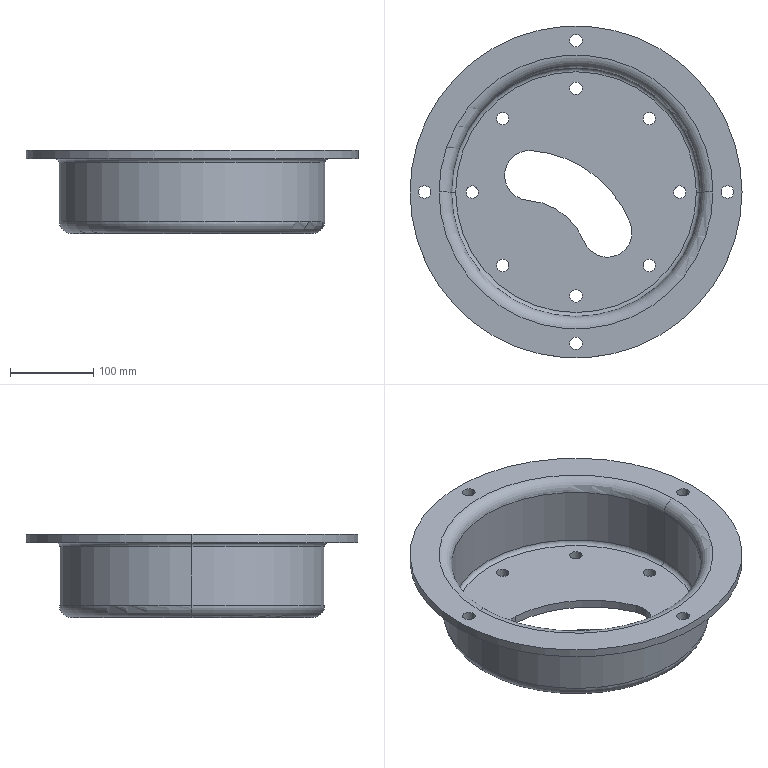Part | SolidWorks | features Fillet 2, ICE 2, Extrusion 1 | 1 solid | 47 faces | box 400 x 400 x 100 mm | volume 1926675 mm3 | cylinder 35 | torus 8 | plane 4 | commonest cylinder face diameters 15 x24 60 x3 300 x2 320 x2 400 x2 160 x1
STEP:
#1=CARTESIAN_POINT('',(-145.,0.,0.));
#2=VERTEX_POINT('',#1);
#3=CARTESIAN_POINT('',(145.,0.,0.));
#4=VERTEX_POINT('',#3);
#5=CARTESIAN_POINT('',(0.,0.,0.));
#6=DIRECTION('',(0.,0.,-1.));
#7=DIRECTION('',(1.,0.,0.));
#8=AXIS2_PLACEMENT_3D('',#5,#6,#7);
#9=CIRCLE('',#8,145.);
#10=EDGE_CURVE('',#2,#4,#9,.T.);
#11=ORIENTED_EDGE('',*,*,#10,.F.);
#12=CARTESIAN_POINT('',(-160.,0.,15.));
#13=VERTEX_POINT('',#12);
#14=CARTESIAN_POINT('',(-145.,0.,15.));
#15=DIRECTION('',(0.,1.,0.));
#16=DIRECTION('',(-1.,0.,0.));
#17=AXIS2_PLACEMENT_3D('',#14,#15,#16);
#18=CIRCLE('',#17,15.);
#19=EDGE_CURVE('',#2,#13,#18,.T.);
#20=ORIENTED_EDGE('',*,*,#19,.T.);
#21=CARTESIAN_POINT('',(160.,0.,15.));
#22=VERTEX_POINT('',#21);
#23=CARTESIAN_POINT('',(0.,0.,15.));
#24=DIRECTION('',(0.,0.,1.));
#25=DIRECTION('',(1.,0.,0.));
#26=AXIS2_PLACEMENT_3D('',#23,#24,#25);
#27=CIRCLE('',#26,160.);
#28=EDGE_CURVE('',#22,#13,#27,.T.);
#29=ORIENTED_EDGE('',*,*,#28,.F.);
#30=CARTESIAN_POINT('',(145.,0.,15.));
#31=DIRECTION('',(0.,-1.,0.));
#32=DIRECTION('',(0.,0.,-1.));
#33=AXIS2_PLACEMENT_3D('',#30,#31,#32);
#34=CIRCLE('',#33,15.);
#35=EDGE_CURVE('',#4,#22,#34,.T.);
#36=ORIENTED_EDGE('',*,*,#35,.F.);
#37=EDGE_LOOP('',(#11,#20,#29,#36));
#38=FACE_OUTER_BOUND('',#37,.T.);
#39=CARTESIAN_POINT('',(0.,0.,15.));
#40=DIRECTION('',(0.,0.,1.));
#41=DIRECTION('',(1.,0.,0.));
#42=AXIS2_PLACEMENT_3D('',#39,#40,#41);
#43=TOROIDAL_SURFACE('',#42,145.,15.);
#44=ADVANCED_FACE('',(#38),#43,.T.);
#45=CARTESIAN_POINT('',(-165.,0.,100.));
#46=VERTEX_POINT('',#45);
#47=CARTESIAN_POINT('',(165.,0.,100.));
#48=VERTEX_POINT('',#47);
#49=CARTESIAN_POINT('',(0.,0.,100.));
#50=DIRECTION('',(0.,0.,-1.));
#51=DIRECTION('',(1.,0.,0.));
#52=AXIS2_PLACEMENT_3D('',#49,#50,#51);
#53=CIRCLE('',#52,165.);
#54=EDGE_CURVE('',#46,#48,#53,.T.);
#55=ORIENTED_EDGE('',*,*,#54,.F.);
#56=CARTESIAN_POINT('',(-150.,0.,85.));
#57=VERTEX_POINT('',#56);
#58=CARTESIAN_POINT('',(-165.,0.,85.));
#59=DIRECTION('',(0.,1.,0.));
#60=DIRECTION('',(-1.,0.,0.));
#61=AXIS2_PLACEMENT_3D('',#58,#59,#60);
#62=CIRCLE('',#61,15.);
#63=EDGE_CURVE('',#46,#57,#62,.T.);
#64=ORIENTED_EDGE('',*,*,#63,.T.);
#65=CARTESIAN_POINT('',(150.,0.,85.));
#66=VERTEX_POINT('',#65);
#67=CARTESIAN_POINT('',(0.,0.,85.));
#68=DIRECTION('',(0.,0.,1.));
#69=DIRECTION('',(1.,0.,0.));
#70=AXIS2_PLACEMENT_3D('',#67,#68,#69);
#71=CIRCLE('',#70,150.);
#72=EDGE_CURVE('',#66,#57,#71,.T.);
#73=ORIENTED_EDGE('',*,*,#72,.F.);
#74=CARTESIAN_POINT('',(165.,0.,85.));
#75=DIRECTION('',(0.,-1.,0.));
#76=DIRECTION('',(0.,0.,-1.));
#77=AXIS2_PLACEMENT_3D('',#74,#75,#76);
#78=CIRCLE('',#77,15.);
#79=EDGE_CURVE('',#48,#66,#78,.T.);
#80=ORIENTED_EDGE('',*,*,#79,.F.);
#81=EDGE_LOOP('',(#55,#64,#73,#80));
#82=FACE_OUTER_BOUND('',#81,.T.);
#83=CARTESIAN_POINT('',(0.,0.,85.));
#84=DIRECTION('',(0.,0.,1.));
#85=DIRECTION('',(1.,0.,0.));
#86=AXIS2_PLACEMENT_3D('',#83,#84,#85);
#87=TOROIDAL_SURFACE('',#86,165.,15.);
#88=ADVANCED_FACE('',(#82),#87,.T.);
#89=CARTESIAN_POINT('',(-145.,0.,10.));
#90=VERTEX_POINT('',#89);
#91=CARTESIAN_POINT('',(145.,0.,10.));
#92=VERTEX_POINT('',#91);
#93=CARTESIAN_POINT('',(0.,0.,10.));
#94=DIRECTION('',(0.,0.,1.));
#95=DIRECTION('',(1.,0.,0.));
#96=AXIS2_PLACEMENT_3D('',#93,#94,#95);
#97=CIRCLE('',#96,145.);
#98=EDGE_CURVE('',#90,#92,#97,.T.);
#99=ORIENTED_EDGE('',*,*,#98,.F.);
#100=CARTESIAN_POINT('',(-150.,0.,15.));
#101=VERTEX_POINT('',#100);
#102=CARTESIAN_POINT('',(-145.,0.,15.));
#103=DIRECTION('',(0.,1.,0.));
#104=DIRECTION('',(-1.,0.,0.));
#105=AXIS2_PLACEMENT_3D('',#102,#103,#104);
#106=CIRCLE('',#105,5.);
#107=EDGE_CURVE('',#90,#101,#106,.T.);
#108=ORIENTED_EDGE('',*,*,#107,.T.);
#109=CARTESIAN_POINT('',(150.,0.,15.));
#110=VERTEX_POINT('',#109);
#111=CARTESIAN_POINT('',(0.,0.,15.));
#112=DIRECTION('',(0.,0.,-1.));
#113=DIRECTION('',(1.,0.,0.));
#114=AXIS2_PLACEMENT_3D('',#111,#112,#113);
#115=CIRCLE('',#114,150.);
#116=EDGE_CURVE('',#110,#101,#115,.T.);
#117=ORIENTED_EDGE('',*,*,#116,.F.);
#118=CARTESIAN_POINT('',(145.,0.,15.));
#119=DIRECTION('',(0.,-1.,0.));
#120=DIRECTION('',(0.,0.,-1.));
#121=AXIS2_PLACEMENT_3D('',#118,#119,#120);
#122=CIRCLE('',#121,5.);
#123=EDGE_CURVE('',#92,#110,#122,.T.);
#124=ORIENTED_EDGE('',*,*,#123,.F.);
#125=EDGE_LOOP('',(#99,#108,#117,#124));
#126=FACE_OUTER_BOUND('',#125,.T.);
#127=CARTESIAN_POINT('',(0.,0.,15.));
#128=DIRECTION('',(0.,0.,1.));
#129=DIRECTION('',(1.,0.,0.));
#130=AXIS2_PLACEMENT_3D('',#127,#128,#129);
#131=TOROIDAL_SURFACE('',#130,145.,5.);
#132=ADVANCED_FACE('',(#126),#131,.F.);
#133=CARTESIAN_POINT('',(-165.,0.,90.));
#134=VERTEX_POINT('',#133);
#135=CARTESIAN_POINT('',(165.,0.,90.));
#136=VERTEX_POINT('',#135);
#137=CARTESIAN_POINT('',(0.,0.,90.));
#138=DIRECTION('',(0.,0.,1.));
#139=DIRECTION('',(1.,0.,0.));
#140=AXIS2_PLACEMENT_3D('',#137,#138,#139);
#141=CIRCLE('',#140,165.);
#142=EDGE_CURVE('',#134,#136,#141,.T.);
#143=ORIENTED_EDGE('',*,*,#142,.F.);
#144=CARTESIAN_POINT('',(-160.,0.,85.));
#145=VERTEX_POINT('',#144);
#146=CARTESIAN_POINT('',(-165.,0.,85.));
#147=DIRECTION('',(0.,1.,0.));
#148=DIRECTION('',(-1.,0.,0.));
#149=AXIS2_PLACEMENT_3D('',#146,#147,#148);
#150=CIRCLE('',#149,5.);
#151=EDGE_CURVE('',#134,#145,#150,.T.);
#152=ORIENTED_EDGE('',*,*,#151,.T.);
#153=CARTESIAN_POINT('',(160.,0.,85.));
#154=VERTEX_POINT('',#153);
#155=CARTESIAN_POINT('',(0.,0.,85.));
#156=DIRECTION('',(0.,0.,-1.));
#157=DIRECTION('',(1.,0.,0.));
#158=AXIS2_PLACEMENT_3D('',#155,#156,#157);
#159=CIRCLE('',#158,160.);
#160=EDGE_CURVE('',#154,#145,#159,.T.);
#161=ORIENTED_EDGE('',*,*,#160,.F.);
#162=CARTESIAN_POINT('',(165.,0.,85.));
#163=DIRECTION('',(0.,-1.,0.));
#164=DIRECTION('',(0.,0.,-1.));
#165=AXIS2_PLACEMENT_3D('',#162,#163,#164);
#166=CIRCLE('',#165,5.);
#167=EDGE_CURVE('',#136,#154,#166,.T.);
#168=ORIENTED_EDGE('',*,*,#167,.F.);
#169=EDGE_LOOP('',(#143,#152,#161,#168));
#170=FACE_OUTER_BOUND('',#169,.T.);
#171=CARTESIAN_POINT('',(0.,0.,85.));
#172=DIRECTION('',(0.,0.,1.));
#173=DIRECTION('',(1.,0.,0.));
#174=AXIS2_PLACEMENT_3D('',#171,#172,#173);
#175=TOROIDAL_SURFACE('',#174,165.,5.);
#176=ADVANCED_FACE('',(#170),#175,.F.);
#177=CARTESIAN_POINT('',(-190.,0.,100.));
#178=VERTEX_POINT('',#177);
#179=CARTESIAN_POINT('',(-175.,0.,100.));
#180=VERTEX_POINT('',#179);
#181=CARTESIAN_POINT('',(-182.5,0.,100.));
#182=DIRECTION('',(0.,0.,1.));
#183=DIRECTION('',(1.,0.,0.));
#184=AXIS2_PLACEMENT_3D('',#181,#182,#183);
#185=CIRCLE('',#184,7.5);
#186=EDGE_CURVE('',#178,#180,#185,.T.);
#187=ORIENTED_EDGE('',*,*,#186,.T.);
#188=CARTESIAN_POINT('',(-175.,0.,90.));
#189=VERTEX_POINT('',#188);
#190=CARTESIAN_POINT('',(-175.,0.,100.));
#191=DIRECTION('',(0.,0.,-1.));
#192=VECTOR('',#191,1000.);
#193=LINE('',#190,#192);
#194=EDGE_CURVE('',#180,#189,#193,.T.);
#195=ORIENTED_EDGE('',*,*,#194,.T.);
#196=CARTESIAN_POINT('',(-190.,0.,90.));
#197=VERTEX_POINT('',#196);
#198=CARTESIAN_POINT('',(-182.5,0.,90.));
#199=DIRECTION('',(0.,0.,1.));
#200=DIRECTION('',(1.,0.,0.));
#201=AXIS2_PLACEMENT_3D('',#198,#199,#200);
#202=CIRCLE('',#201,7.5);
#203=EDGE_CURVE('',#197,#189,#202,.T.);
#204=ORIENTED_EDGE('',*,*,#203,.F.);
#205=CARTESIAN_POINT('',(-190.,0.,100.));
#206=DIRECTION('',(0.,0.,-1.));
#207=VECTOR('',#206,1000.);
#208=LINE('',#205,#207);
#209=EDGE_CURVE('',#178,#197,#208,.T.);
#210=ORIENTED_EDGE('',*,*,#209,.F.);
#211=EDGE_LOOP('',(#187,#195,#204,#210));
#212=FACE_OUTER_BOUND('',#211,.T.);
#213=CARTESIAN_POINT('',(-182.5,0.,100.));
#214=DIRECTION('',(0.,0.,-1.));
#215=DIRECTION('',(-1.,0.,0.));
#216=AXIS2_PLACEMENT_3D('',#213,#214,#215);
#217=CYLINDRICAL_SURFACE('',#216,7.5);
#218=ADVANCED_FACE('',(#212),#217,.F.);
#219=CARTESIAN_POINT('',(-7.5,-182.5,100.));
#220=VERTEX_POINT('',#219);
#221=CARTESIAN_POINT('',(7.5,-182.5,100.));
#222=VERTEX_POINT('',#221);
#223=CARTESIAN_POINT('',(0.,-182.5,100.));
#224=DIRECTION('',(0.,0.,1.));
#225=DIRECTION('',(1.,0.,0.));
#226=AXIS2_PLACEMENT_3D('',#223,#224,#225);
#227=CIRCLE('',#226,7.5);
#228=EDGE_CURVE('',#220,#222,#227,.T.);
#229=ORIENTED_EDGE('',*,*,#228,.T.);
#230=CARTESIAN_POINT('',(7.5,-182.5,90.));
#231=VERTEX_POINT('',#230);
#232=CARTESIAN_POINT('',(7.5,-182.5,100.));
#233=DIRECTION('',(0.,0.,-1.));
#234=VECTOR('',#233,1000.);
#235=LINE('',#232,#234);
#236=EDGE_CURVE('',#222,#231,#235,.T.);
#237=ORIENTED_EDGE('',*,*,#236,.T.);
#238=CARTESIAN_POINT('',(-7.5,-182.5,90.));
#239=VERTEX_POINT('',#238);
#240=CARTESIAN_POINT('',(0.,-182.5,90.));
#241=DIRECTION('',(0.,0.,1.));
#242=DIRECTION('',(1.,0.,0.));
#243=AXIS2_PLACEMENT_3D('',#240,#241,#242);
#244=CIRCLE('',#243,7.5);
#245=EDGE_CURVE('',#239,#231,#244,.T.);
#246=ORIENTED_EDGE('',*,*,#245,.F.);
#247=CARTESIAN_POINT('',(-7.5,-182.5,100.));
#248=DIRECTION('',(0.,0.,-1.));
#249=VECTOR('',#248,1000.);
#250=LINE('',#247,#249);
#251=EDGE_CURVE('',#220,#239,#250,.T.);
#252=ORIENTED_EDGE('',*,*,#251,.F.);
#253=EDGE_LOOP('',(#229,#237,#246,#252));
#254=FACE_OUTER_BOUND('',#253,.T.);
#255=CARTESIAN_POINT('',(0.,-182.5,100.));
#256=DIRECTION('',(0.,0.,-1.));
#257=DIRECTION('',(-1.,0.,0.));
#258=AXIS2_PLACEMENT_3D('',#255,#256,#257);
#259=CYLINDRICAL_SURFACE('',#258,7.5);
#260=ADVANCED_FACE('',(#254),#259,.F.);
#261=CARTESIAN_POINT('',(175.,0.,100.));
#262=VERTEX_POINT('',#261);
#263=CARTESIAN_POINT('',(190.,0.,100.));
#264=VERTEX_POINT('',#263);
#265=CARTESIAN_POINT('',(182.5,0.,100.));
#266=DIRECTION('',(0.,0.,1.));
#267=DIRECTION('',(1.,0.,0.));
#268=AXIS2_PLACEMENT_3D('',#265,#266,#267);
#269=CIRCLE('',#268,7.5);
#270=EDGE_CURVE('',#262,#264,#269,.T.);
#271=ORIENTED_EDGE('',*,*,#270,.T.);
#272=CARTESIAN_POINT('',(190.,0.,90.));
#273=VERTEX_POINT('',#272);
#274=CARTESIAN_POINT('',(190.,0.,100.));
#275=DIRECTION('',(0.,0.,-1.));
#276=VECTOR('',#275,1000.);
#277=LINE('',#274,#276);
#278=EDGE_CURVE('',#264,#273,#277,.T.);
#279=ORIENTED_EDGE('',*,*,#278,.T.);
#280=CARTESIAN_POINT('',(175.,0.,90.));
#281=VERTEX_POINT('',#280);
#282=CARTESIAN_POINT('',(182.5,0.,90.));
#283=DIRECTION('',(0.,0.,1.));
#284=DIRECTION('',(1.,0.,0.));
#285=AXIS2_PLACEMENT_3D('',#282,#283,#284);
#286=CIRCLE('',#285,7.5);
#287=EDGE_CURVE('',#281,#273,#286,.T.);
#288=ORIENTED_EDGE('',*,*,#287,.F.);
#289=CARTESIAN_POINT('',(175.,0.,100.));
#290=DIRECTION('',(0.,0.,-1.));
#291=VECTOR('',#290,1000.);
#292=LINE('',#289,#291);
#293=EDGE_CURVE('',#262,#281,#292,.T.);
#294=ORIENTED_EDGE('',*,*,#293,.F.);
#295=EDGE_LOOP('',(#271,#279,#288,#294));
#296=FACE_OUTER_BOUND('',#295,.T.);
#297=CARTESIAN_POINT('',(182.5,0.,100.));
#298=DIRECTION('',(0.,0.,-1.));
#299=DIRECTION('',(-1.,0.,0.));
#300=AXIS2_PLACEMENT_3D('',#297,#298,#299);
#301=CYLINDRICAL_SURFACE('',#300,7.5);
#302=ADVANCED_FACE('',(#296),#301,.F.);
#303=CARTESIAN_POINT('',(-7.5,182.5,100.));
#304=VERTEX_POINT('',#303);
#305=CARTESIAN_POINT('',(7.5,182.5,100.));
#306=VERTEX_POINT('',#305);
#307=CARTESIAN_POINT('',(0.,182.5,100.));
#308=DIRECTION('',(0.,0.,1.));
#309=DIRECTION('',(1.,0.,0.));
#310=AXIS2_PLACEMENT_3D('',#307,#308,#309);
#311=CIRCLE('',#310,7.5);
#312=EDGE_CURVE('',#304,#306,#311,.T.);
#313=ORIENTED_EDGE('',*,*,#312,.T.);
#314=CARTESIAN_POINT('',(7.5,182.5,90.));
#315=VERTEX_POINT('',#314);
#316=CARTESIAN_POINT('',(7.5,182.5,100.));
#317=DIRECTION('',(0.,0.,-1.));
#318=VECTOR('',#317,1000.);
#319=LINE('',#316,#318);
#320=EDGE_CURVE('',#306,#315,#319,.T.);
#321=ORIENTED_EDGE('',*,*,#320,.T.);
#322=CARTESIAN_POINT('',(-7.5,182.5,90.));
#323=VERTEX_POINT('',#322);
#324=CARTESIAN_POINT('',(0.,182.5,90.));
#325=DIRECTION('',(0.,0.,1.));
#326=DIRECTION('',(1.,0.,0.));
#327=AXIS2_PLACEMENT_3D('',#324,#325,#326);
#328=CIRCLE('',#327,7.5);
#329=EDGE_CURVE('',#323,#315,#328,.T.);
#330=ORIENTED_EDGE('',*,*,#329,.F.);
#331=CARTESIAN_POINT('',(-7.5,182.5,100.));
#332=DIRECTION('',(0.,0.,-1.));
#333=VECTOR('',#332,1000.);
#334=LINE('',#331,#333);
#335=EDGE_CURVE('',#304,#323,#334,.T.);
#336=ORIENTED_EDGE('',*,*,#335,.F.);
#337=EDGE_LOOP('',(#313,#321,#330,#336));
#338=FACE_OUTER_BOUND('',#337,.T.);
#339=CARTESIAN_POINT('',(0.,182.5,100.));
#340=DIRECTION('',(0.,0.,-1.));
#341=DIRECTION('',(-1.,0.,0.));
#342=AXIS2_PLACEMENT_3D('',#339,#340,#341);
#343=CYLINDRICAL_SURFACE('',#342,7.5);
#344=ADVANCED_FACE('',(#338),#343,.F.);
#345=CARTESIAN_POINT('',(200.,0.,100.));
#346=VERTEX_POINT('',#345);
#347=CARTESIAN_POINT('',(-200.,0.,100.));
#348=VERTEX_POINT('',#347);
#349=CARTESIAN_POINT('',(0.,0.,100.));
#350=DIRECTION('',(0.,0.,1.));
#351=DIRECTION('',(1.,0.,0.));
#352=AXIS2_PLACEMENT_3D('',#349,#350,#351);
#353=CIRCLE('',#352,200.);
#354=EDGE_CURVE('',#346,#348,#353,.T.);
#355=ORIENTED_EDGE('',*,*,#354,.F.);
#356=CARTESIAN_POINT('',(200.,0.,90.));
#357=VERTEX_POINT('',#356);
#358=CARTESIAN_POINT('',(200.,0.,100.));
#359=DIRECTION('',(0.,0.,-1.));
#360=VECTOR('',#359,1000.);
#361=LINE('',#358,#360);
#362=EDGE_CURVE('',#346,#357,#361,.T.);
#363=ORIENTED_EDGE('',*,*,#362,.T.);
#364=CARTESIAN_POINT('',(-200.,0.,90.));
#365=VERTEX_POINT('',#364);
#366=CARTESIAN_POINT('',(0.,0.,90.));
#367=DIRECTION('',(0.,0.,1.));
#368=DIRECTION('',(1.,0.,0.));
#369=AXIS2_PLACEMENT_3D('',#366,#367,#368);
#370=CIRCLE('',#369,200.);
#371=EDGE_CURVE('',#357,#365,#370,.T.);
#372=ORIENTED_EDGE('',*,*,#371,.T.);
#373=CARTESIAN_POINT('',(-200.,0.,100.));
#374=DIRECTION('',(0.,0.,-1.));
#375=VECTOR('',#374,1000.);
#376=LINE('',#373,#375);
#377=EDGE_CURVE('',#348,#365,#376,.T.);
#378=ORIENTED_EDGE('',*,*,#377,.F.);
#379=EDGE_LOOP('',(#355,#363,#372,#378));
#380=FACE_OUTER_BOUND('',#379,.T.);
#381=CARTESIAN_POINT('',(0.,0.,100.));
#382=DIRECTION('',(0.,0.,-1.));
#383=DIRECTION('',(-1.,0.,0.));
#384=AXIS2_PLACEMENT_3D('',#381,#382,#383);
#385=CYLINDRICAL_SURFACE('',#384,200.);
#386=ADVANCED_FACE('',(#380),#385,.T.);
#387=CARTESIAN_POINT('',(0.,0.,85.));
#388=DIRECTION('',(0.,0.,1.));
#389=DIRECTION('',(1.,0.,0.));
#390=AXIS2_PLACEMENT_3D('',#387,#388,#389);
#391=CIRCLE('',#390,150.);
#392=EDGE_CURVE('',#57,#66,#391,.T.);
#393=ORIENTED_EDGE('',*,*,#392,.T.);
#394=CARTESIAN_POINT('',(150.,0.,90.));
#395=DIRECTION('',(0.,0.,-1.));
#396=VECTOR('',#395,1000.);
#397=LINE('',#394,#396);
#398=EDGE_CURVE('',#66,#110,#397,.T.);
#399=ORIENTED_EDGE('',*,*,#398,.T.);
#400=ORIENTED_EDGE('',*,*,#116,.T.);
#401=CARTESIAN_POINT('',(-150.,0.,90.));
#402=DIRECTION('',(0.,0.,-1.));
#403=VECTOR('',#402,1000.);
#404=LINE('',#401,#403);
#405=EDGE_CURVE('',#57,#101,#404,.T.);
#406=ORIENTED_EDGE('',*,*,#405,.F.);
#407=EDGE_LOOP('',(#393,#399,#400,#406));
#408=FACE_OUTER_BOUND('',#407,.T.);
#409=CARTESIAN_POINT('',(0.,0.,90.));
#410=DIRECTION('',(0.,0.,-1.));
#411=DIRECTION('',(-1.,0.,0.));
#412=AXIS2_PLACEMENT_3D('',#409,#410,#411);
#413=CYLINDRICAL_SURFACE('',#412,150.);
#414=ADVANCED_FACE('',(#408),#413,.F.);
#415=CARTESIAN_POINT('',(-53.803,50.038,10.));
#416=VERTEX_POINT('',#415);
#417=CARTESIAN_POINT('',(-86.087,20.125,10.));
#418=VERTEX_POINT('',#417);
#419=CARTESIAN_POINT('',(-56.087,20.125,10.));
#420=DIRECTION('',(0.,0.,1.));
#421=DIRECTION('',(1.,0.,0.));
#422=AXIS2_PLACEMENT_3D('',#419,#420,#421);
#423=CIRCLE('',#422,30.);
#424=EDGE_CURVE('',#416,#418,#423,.T.);
#425=ORIENTED_EDGE('',*,*,#424,.T.);
#426=CARTESIAN_POINT('',(-86.087,20.125,0.));
#427=VERTEX_POINT('',#426);
#428=CARTESIAN_POINT('',(-86.087,20.125,10.));
#429=DIRECTION('',(0.,0.,-1.));
#430=VECTOR('',#429,1000.);
#431=LINE('',#428,#430);
#432=EDGE_CURVE('',#418,#427,#431,.T.);
#433=ORIENTED_EDGE('',*,*,#432,.T.);
#434=CARTESIAN_POINT('',(-53.803,50.038,0.));
#435=VERTEX_POINT('',#434);
#436=CARTESIAN_POINT('',(-56.087,20.125,0.));
#437=DIRECTION('',(0.,0.,1.));
#438=DIRECTION('',(1.,0.,0.));
#439=AXIS2_PLACEMENT_3D('',#436,#437,#438);
#440=CIRCLE('',#439,30.);
#441=EDGE_CURVE('',#435,#427,#440,.T.);
#442=ORIENTED_EDGE('',*,*,#441,.F.);
#443=CARTESIAN_POINT('',(-53.803,50.038,10.));
#444=DIRECTION('',(0.,0.,-1.));
#445=VECTOR('',#444,1000.);
#446=LINE('',#443,#445);
#447=EDGE_CURVE('',#416,#435,#446,.T.);
#448=ORIENTED_EDGE('',*,*,#447,.F.);
#449=EDGE_LOOP('',(#425,#433,#442,#448));
#450=FACE_OUTER_BOUND('',#449,.T.);
#451=CARTESIAN_POINT('',(-56.087,20.125,10.));
#452=DIRECTION('',(0.,0.,-1.));
#453=DIRECTION('',(-1.,0.,0.));
#454=AXIS2_PLACEMENT_3D('',#451,#452,#453);
#455=CYLINDRICAL_SURFACE('',#454,30.);
#456=ADVANCED_FACE('',(#450),#455,.F.);
#457=CARTESIAN_POINT('',(-95.888,88.388,10.));
#458=VERTEX_POINT('',#457);
#459=CARTESIAN_POINT('',(-80.888,88.388,10.));
#460=VERTEX_POINT('',#459);
#461=CARTESIAN_POINT('',(-88.388,88.388,10.));
#462=DIRECTION('',(0.,0.,1.));
#463=DIRECTION('',(1.,0.,0.));
#464=AXIS2_PLACEMENT_3D('',#461,#462,#463);
#465=CIRCLE('',#464,7.5);
#466=EDGE_CURVE('',#458,#460,#465,.T.);
#467=ORIENTED_EDGE('',*,*,#466,.T.);
#468=CARTESIAN_POINT('',(-80.888,88.388,0.));
#469=VERTEX_POINT('',#468);
#470=CARTESIAN_POINT('',(-80.888,88.388,10.));
#471=DIRECTION('',(0.,0.,-1.));
#472=VECTOR('',#471,1000.);
#473=LINE('',#470,#472);
#474=EDGE_CURVE('',#460,#469,#473,.T.);
#475=ORIENTED_EDGE('',*,*,#474,.T.);
#476=CARTESIAN_POINT('',(-95.888,88.388,0.));
#477=VERTEX_POINT('',#476);
#478=CARTESIAN_POINT('',(-88.388,88.388,0.));
#479=DIRECTION('',(0.,0.,1.));
#480=DIRECTION('',(1.,0.,0.));
#481=AXIS2_PLACEMENT_3D('',#478,#479,#480);
#482=CIRCLE('',#481,7.5);
#483=EDGE_CURVE('',#477,#469,#482,.T.);
#484=ORIENTED_EDGE('',*,*,#483,.F.);
#485=CARTESIAN_POINT('',(-95.888,88.388,10.));
#486=DIRECTION('',(0.,0.,-1.));
#487=VECTOR('',#486,1000.);
#488=LINE('',#485,#487);
#489=EDGE_CURVE('',#458,#477,#488,.T.);
#490=ORIENTED_EDGE('',*,*,#489,.F.);
#491=EDGE_LOOP('',(#467,#475,#484,#490));
#492=FACE_OUTER_BOUND('',#491,.T.);
#493=CARTESIAN_POINT('',(-88.388,88.388,10.));
#494=DIRECTION('',(0.,0.,-1.));
#495=DIRECTION('',(-1.,0.,0.));
#496=AXIS2_PLACEMENT_3D('',#493,#494,#495);
#497=CYLINDRICAL_SURFACE('',#496,7.5);
#498=ADVANCED_FACE('',(#492),#497,.F.);
#499=CARTESIAN_POINT('',(-132.5,0.,10.));
#500=VERTEX_POINT('',#499);
#501=CARTESIAN_POINT('',(-117.5,0.,10.));
#502=VERTEX_POINT('',#501);
#503=CARTESIAN_POINT('',(-125.,0.,10.));
#504=DIRECTION('',(0.,0.,1.));
#505=DIRECTION('',(1.,0.,0.));
#506=AXIS2_PLACEMENT_3D('',#503,#504,#505);
#507=CIRCLE('',#506,7.5);
#508=EDGE_CURVE('',#500,#502,#507,.T.);
#509=ORIENTED_EDGE('',*,*,#508,.T.);
#510=CARTESIAN_POINT('',(-117.5,0.,0.));
#511=VERTEX_POINT('',#510);
#512=CARTESIAN_POINT('',(-117.5,0.,10.));
#513=DIRECTION('',(0.,0.,-1.));
#514=VECTOR('',#513,1000.);
#515=LINE('',#512,#514);
#516=EDGE_CURVE('',#502,#511,#515,.T.);
#517=ORIENTED_EDGE('',*,*,#516,.T.);
#518=CARTESIAN_POINT('',(-132.5,0.,0.));
#519=VERTEX_POINT('',#518);
#520=CARTESIAN_POINT('',(-125.,0.,0.));
#521=DIRECTION('',(0.,0.,1.));
#522=DIRECTION('',(1.,0.,0.));
#523=AXIS2_PLACEMENT_3D('',#520,#521,#522);
#524=CIRCLE('',#523,7.5);
#525=EDGE_CURVE('',#519,#511,#524,.T.);
#526=ORIENTED_EDGE('',*,*,#525,.F.);
#527=CARTESIAN_POINT('',(-132.5,0.,10.));
#528=DIRECTION('',(0.,0.,-1.));
#529=VECTOR('',#528,1000.);
#530=LINE('',#527,#529);
#531=EDGE_CURVE('',#500,#519,#530,.T.);
#532=ORIENTED_EDGE('',*,*,#531,.F.);
#533=EDGE_LOOP('',(#509,#517,#526,#532));
#534=FACE_OUTER_BOUND('',#533,.T.);
#535=CARTESIAN_POINT('',(-125.,0.,10.));
#536=DIRECTION('',(0.,0.,-1.));
#537=DIRECTION('',(-1.,0.,0.));
#538=AXIS2_PLACEMENT_3D('',#535,#536,#537);
#539=CYLINDRICAL_SURFACE('',#538,7.5);
#540=ADVANCED_FACE('',(#534),#539,.F.);
#541=CARTESIAN_POINT('',(-95.888,-88.388,10.));
#542=VERTEX_POINT('',#541);
#543=CARTESIAN_POINT('',(-80.888,-88.388,10.));
#544=VERTEX_POINT('',#543);
#545=CARTESIAN_POINT('',(-88.388,-88.388,10.));
#546=DIRECTION('',(0.,0.,1.));
#547=DIRECTION('',(1.,0.,0.));
#548=AXIS2_PLACEMENT_3D('',#545,#546,#547);
#549=CIRCLE('',#548,7.5);
#550=EDGE_CURVE('',#542,#544,#549,.T.);
#551=ORIENTED_EDGE('',*,*,#550,.T.);
#552=CARTESIAN_POINT('',(-80.888,-88.388,0.));
#553=VERTEX_POINT('',#552);
#554=CARTESIAN_POINT('',(-80.888,-88.388,10.));
#555=DIRECTION('',(0.,0.,-1.));
#556=VECTOR('',#555,1000.);
#557=LINE('',#554,#556);
#558=EDGE_CURVE('',#544,#553,#557,.T.);
#559=ORIENTED_EDGE('',*,*,#558,.T.);
#560=CARTESIAN_POINT('',(-95.888,-88.388,0.));
#561=VERTEX_POINT('',#560);
#562=CARTESIAN_POINT('',(-88.388,-88.388,0.));
#563=DIRECTION('',(0.,0.,1.));
#564=DIRECTION('',(1.,0.,0.));
#565=AXIS2_PLACEMENT_3D('',#562,#563,#564);
#566=CIRCLE('',#565,7.5);
#567=EDGE_CURVE('',#561,#553,#566,.T.);
#568=ORIENTED_EDGE('',*,*,#567,.F.);
#569=CARTESIAN_POINT('',(-95.888,-88.388,10.));
#570=DIRECTION('',(0.,0.,-1.));
#571=VECTOR('',#570,1000.);
#572=LINE('',#569,#571);
#573=EDGE_CURVE('',#542,#561,#572,.T.);
#574=ORIENTED_EDGE('',*,*,#573,.F.);
#575=EDGE_LOOP('',(#551,#559,#568,#574));
#576=FACE_OUTER_BOUND('',#575,.T.);
#577=CARTESIAN_POINT('',(-88.388,-88.388,10.));
#578=DIRECTION('',(0.,0.,-1.));
#579=DIRECTION('',(-1.,0.,0.));
#580=AXIS2_PLACEMENT_3D('',#577,#578,#579);
#581=CYLINDRICAL_SURFACE('',#580,7.5);
#582=ADVANCED_FACE('',(#576),#581,.F.);
#583=CARTESIAN_POINT('',(-7.5,-125.,10.));
#584=VERTEX_POINT('',#583);
#585=CARTESIAN_POINT('',(7.5,-125.,10.));
#586=VERTEX_POINT('',#585);
#587=CARTESIAN_POINT('',(0.,-125.,10.));
#588=DIRECTION('',(0.,0.,1.));
#589=DIRECTION('',(1.,0.,0.));
#590=AXIS2_PLACEMENT_3D('',#587,#588,#589);
#591=CIRCLE('',#590,7.5);
#592=EDGE_CURVE('',#584,#586,#591,.T.);
#593=ORIENTED_EDGE('',*,*,#592,.T.);
#594=CARTESIAN_POINT('',(7.5,-125.,0.));
#595=VERTEX_POINT('',#594);
#596=CARTESIAN_POINT('',(7.5,-125.,10.));
#597=DIRECTION('',(0.,0.,-1.));
#598=VECTOR('',#597,1000.);
#599=LINE('',#596,#598);
#600=EDGE_CURVE('',#586,#595,#599,.T.);
#601=ORIENTED_EDGE('',*,*,#600,.T.);
#602=CARTESIAN_POINT('',(-7.5,-125.,0.));
#603=VERTEX_POINT('',#602);
#604=CARTESIAN_POINT('',(0.,-125.,0.));
#605=DIRECTION('',(0.,0.,1.));
#606=DIRECTION('',(1.,0.,0.));
#607=AXIS2_PLACEMENT_3D('',#604,#605,#606);
#608=CIRCLE('',#607,7.5);
#609=EDGE_CURVE('',#603,#595,#608,.T.);
#610=ORIENTED_EDGE('',*,*,#609,.F.);
#611=CARTESIAN_POINT('',(-7.5,-125.,10.));
#612=DIRECTION('',(0.,0.,-1.));
#613=VECTOR('',#612,1000.);
#614=LINE('',#611,#613);
#615=EDGE_CURVE('',#584,#603,#614,.T.);
#616=ORIENTED_EDGE('',*,*,#615,.F.);
#617=EDGE_LOOP('',(#593,#601,#610,#616));
#618=FACE_OUTER_BOUND('',#617,.T.);
#619=CARTESIAN_POINT('',(0.,-125.,10.));
#620=DIRECTION('',(0.,0.,-1.));
#621=DIRECTION('',(-1.,0.,0.));
#622=AXIS2_PLACEMENT_3D('',#619,#620,#621);
#623=CYLINDRICAL_SURFACE('',#622,7.5);
#624=ADVANCED_FACE('',(#618),#623,.F.);
#625=CARTESIAN_POINT('',(80.888,-88.388,10.));
#626=VERTEX_POINT('',#625);
#627=CARTESIAN_POINT('',(95.888,-88.388,10.));
#628=VERTEX_POINT('',#627);
#629=CARTESIAN_POINT('',(88.388,-88.388,10.));
#630=DIRECTION('',(0.,0.,1.));
#631=DIRECTION('',(1.,0.,0.));
#632=AXIS2_PLACEMENT_3D('',#629,#630,#631);
#633=CIRCLE('',#632,7.5);
#634=EDGE_CURVE('',#626,#628,#633,.T.);
#635=ORIENTED_EDGE('',*,*,#634,.T.);
#636=CARTESIAN_POINT('',(95.888,-88.388,0.));
#637=VERTEX_POINT('',#636);
#638=CARTESIAN_POINT('',(95.888,-88.388,10.));
#639=DIRECTION('',(0.,0.,-1.));
#640=VECTOR('',#639,1000.);
#641=LINE('',#638,#640);
#642=EDGE_CURVE('',#628,#637,#641,.T.);
#643=ORIENTED_EDGE('',*,*,#642,.T.);
#644=CARTESIAN_POINT('',(80.888,-88.388,0.));
#645=VERTEX_POINT('',#644);
#646=CARTESIAN_POINT('',(88.388,-88.388,0.));
#647=DIRECTION('',(0.,0.,1.));
#648=DIRECTION('',(1.,0.,0.));
#649=AXIS2_PLACEMENT_3D('',#646,#647,#648);
#650=CIRCLE('',#649,7.5);
#651=EDGE_CURVE('',#645,#637,#650,.T.);
#652=ORIENTED_EDGE('',*,*,#651,.F.);
#653=CARTESIAN_POINT('',(80.888,-88.388,10.));
#654=DIRECTION('',(0.,0.,-1.));
#655=VECTOR('',#654,1000.);
#656=LINE('',#653,#655);
#657=EDGE_CURVE('',#626,#645,#656,.T.);
#658=ORIENTED_EDGE('',*,*,#657,.F.);
#659=EDGE_LOOP('',(#635,#643,#652,#658));
#660=FACE_OUTER_BOUND('',#659,.T.);
#661=CARTESIAN_POINT('',(88.388,-88.388,10.));
#662=DIRECTION('',(0.,0.,-1.));
#663=DIRECTION('',(-1.,0.,0.));
#664=AXIS2_PLACEMENT_3D('',#661,#662,#663);
#665=CYLINDRICAL_SURFACE('',#664,7.5);
#666=ADVANCED_FACE('',(#660),#665,.F.);
#667=CARTESIAN_POINT('',(117.5,0.,10.));
#668=VERTEX_POINT('',#667);
#669=CARTESIAN_POINT('',(132.5,0.,10.));
#670=VERTEX_POINT('',#669);
#671=CARTESIAN_POINT('',(125.,0.,10.));
#672=DIRECTION('',(0.,0.,1.));
#673=DIRECTION('',(1.,0.,0.));
#674=AXIS2_PLACEMENT_3D('',#671,#672,#673);
#675=CIRCLE('',#674,7.5);
#676=EDGE_CURVE('',#668,#670,#675,.T.);
#677=ORIENTED_EDGE('',*,*,#676,.T.);
#678=CARTESIAN_POINT('',(132.5,0.,0.));
#679=VERTEX_POINT('',#678);
#680=CARTESIAN_POINT('',(132.5,0.,10.));
#681=DIRECTION('',(0.,0.,-1.));
#682=VECTOR('',#681,1000.);
#683=LINE('',#680,#682);
#684=EDGE_CURVE('',#670,#679,#683,.T.);
#685=ORIENTED_EDGE('',*,*,#684,.T.);
#686=CARTESIAN_POINT('',(117.5,0.,0.));
#687=VERTEX_POINT('',#686);
#688=CARTESIAN_POINT('',(125.,0.,0.));
#689=DIRECTION('',(0.,0.,1.));
#690=DIRECTION('',(1.,0.,0.));
#691=AXIS2_PLACEMENT_3D('',#688,#689,#690);
#692=CIRCLE('',#691,7.5);
#693=EDGE_CURVE('',#687,#679,#692,.T.);
#694=ORIENTED_EDGE('',*,*,#693,.F.);
#695=CARTESIAN_POINT('',(117.5,0.,10.));
#696=DIRECTION('',(0.,0.,-1.));
#697=VECTOR('',#696,1000.);
#698=LINE('',#695,#697);
#699=EDGE_CURVE('',#668,#687,#698,.T.);
#700=ORIENTED_EDGE('',*,*,#699,.F.);
#701=EDGE_LOOP('',(#677,#685,#694,#700));
#702=FACE_OUTER_BOUND('',#701,.T.);
#703=CARTESIAN_POINT('',(125.,0.,10.));
#704=DIRECTION('',(0.,0.,-1.));
#705=DIRECTION('',(-1.,0.,0.));
#706=AXIS2_PLACEMENT_3D('',#703,#704,#705);
#707=CYLINDRICAL_SURFACE('',#706,7.5);
#708=ADVANCED_FACE('',(#702),#707,.F.);
#709=CARTESIAN_POINT('',(80.888,88.388,10.));
#710=VERTEX_POINT('',#709);
#711=CARTESIAN_POINT('',(95.888,88.388,10.));
#712=VERTEX_POINT('',#711);
#713=CARTESIAN_POINT('',(88.388,88.388,10.));
#714=DIRECTION('',(0.,0.,1.));
#715=DIRECTION('',(1.,0.,0.));
#716=AXIS2_PLACEMENT_3D('',#713,#714,#715);
#717=CIRCLE('',#716,7.5);
#718=EDGE_CURVE('',#710,#712,#717,.T.);
#719=ORIENTED_EDGE('',*,*,#718,.T.);
#720=CARTESIAN_POINT('',(95.888,88.388,0.));
#721=VERTEX_POINT('',#720);
#722=CARTESIAN_POINT('',(95.888,88.388,10.));
#723=DIRECTION('',(0.,0.,-1.));
#724=VECTOR('',#723,1000.);
#725=LINE('',#722,#724);
#726=EDGE_CURVE('',#712,#721,#725,.T.);
#727=ORIENTED_EDGE('',*,*,#726,.T.);
#728=CARTESIAN_POINT('',(80.888,88.388,0.));
#729=VERTEX_POINT('',#728);
#730=CARTESIAN_POINT('',(88.388,88.388,0.));
#731=DIRECTION('',(0.,0.,1.));
#732=DIRECTION('',(1.,0.,0.));
#733=AXIS2_PLACEMENT_3D('',#730,#731,#732);
#734=CIRCLE('',#733,7.5);
#735=EDGE_CURVE('',#729,#721,#734,.T.);
#736=ORIENTED_EDGE('',*,*,#735,.F.);
#737=CARTESIAN_POINT('',(80.888,88.388,10.));
#738=DIRECTION('',(0.,0.,-1.));
#739=VECTOR('',#738,1000.);
#740=LINE('',#737,#739);
#741=EDGE_CURVE('',#710,#729,#740,.T.);
#742=ORIENTED_EDGE('',*,*,#741,.F.);
#743=EDGE_LOOP('',(#719,#727,#736,#742));
#744=FACE_OUTER_BOUND('',#743,.T.);
#745=CARTESIAN_POINT('',(88.388,88.388,10.));
#746=DIRECTION('',(0.,0.,-1.));
#747=DIRECTION('',(-1.,0.,0.));
#748=AXIS2_PLACEMENT_3D('',#745,#746,#747);
#749=CYLINDRICAL_SURFACE('',#748,7.5);
#750=ADVANCED_FACE('',(#744),#749,.F.);
#751=CARTESIAN_POINT('',(-7.5,125.,10.));
#752=VERTEX_POINT('',#751);
#753=CARTESIAN_POINT('',(7.5,125.,10.));
#754=VERTEX_POINT('',#753);
#755=CARTESIAN_POINT('',(0.,125.,10.));
#756=DIRECTION('',(0.,0.,1.));
#757=DIRECTION('',(1.,0.,0.));
#758=AXIS2_PLACEMENT_3D('',#755,#756,#757);
#759=CIRCLE('',#758,7.5);
#760=EDGE_CURVE('',#752,#754,#759,.T.);
#761=ORIENTED_EDGE('',*,*,#760,.T.);
#762=CARTESIAN_POINT('',(7.5,125.,0.));
#763=VERTEX_POINT('',#762);
#764=CARTESIAN_POINT('',(7.5,125.,10.));
#765=DIRECTION('',(0.,0.,-1.));
#766=VECTOR('',#765,1000.);
#767=LINE('',#764,#766);
#768=EDGE_CURVE('',#754,#763,#767,.T.);
#769=ORIENTED_EDGE('',*,*,#768,.T.);
#770=CARTESIAN_POINT('',(-7.5,125.,0.));
#771=VERTEX_POINT('',#770);
#772=CARTESIAN_POINT('',(0.,125.,0.));
#773=DIRECTION('',(0.,0.,1.));
#774=DIRECTION('',(1.,0.,0.));
#775=AXIS2_PLACEMENT_3D('',#772,#773,#774);
#776=CIRCLE('',#775,7.5);
#777=EDGE_CURVE('',#771,#763,#776,.T.);
#778=ORIENTED_EDGE('',*,*,#777,.F.);
#779=CARTESIAN_POINT('',(-7.5,125.,10.));
#780=DIRECTION('',(0.,0.,-1.));
#781=VECTOR('',#780,1000.);
#782=LINE('',#779,#781);
#783=EDGE_CURVE('',#752,#771,#782,.T.);
#784=ORIENTED_EDGE('',*,*,#783,.F.);
#785=EDGE_LOOP('',(#761,#769,#778,#784));
#786=FACE_OUTER_BOUND('',#785,.T.);
#787=CARTESIAN_POINT('',(0.,125.,10.));
#788=DIRECTION('',(0.,0.,-1.));
#789=DIRECTION('',(-1.,0.,0.));
#790=AXIS2_PLACEMENT_3D('',#787,#788,#789);
#791=CYLINDRICAL_SURFACE('',#790,7.5);
#792=ADVANCED_FACE('',(#786),#791,.F.);
#793=CARTESIAN_POINT('',(0.,0.,85.));
#794=DIRECTION('',(0.,0.,-1.));
#795=DIRECTION('',(1.,0.,0.));
#796=AXIS2_PLACEMENT_3D('',#793,#794,#795);
#797=CIRCLE('',#796,160.);
#798=EDGE_CURVE('',#145,#154,#797,.T.);
#799=ORIENTED_EDGE('',*,*,#798,.T.);
#800=CARTESIAN_POINT('',(160.,0.,10.));
#801=DIRECTION('',(0.,0.,-1.));
#802=VECTOR('',#801,1000.);
#803=LINE('',#800,#802);
#804=EDGE_CURVE('',#154,#22,#803,.T.);
#805=ORIENTED_EDGE('',*,*,#804,.T.);
#806=ORIENTED_EDGE('',*,*,#28,.T.);
#807=CARTESIAN_POINT('',(-160.,0.,10.));
#808=DIRECTION('',(0.,0.,-1.));
#809=VECTOR('',#808,1000.);
#810=LINE('',#807,#809);
#811=EDGE_CURVE('',#145,#13,#810,.T.);
#812=ORIENTED_EDGE('',*,*,#811,.F.);
#813=EDGE_LOOP('',(#799,#805,#806,#812));
#814=FACE_OUTER_BOUND('',#813,.T.);
#815=CARTESIAN_POINT('',(0.,0.,10.));
#816=DIRECTION('',(0.,0.,-1.));
#817=DIRECTION('',(-1.,0.,0.));
#818=AXIS2_PLACEMENT_3D('',#815,#816,#817);
#819=CYLINDRICAL_SURFACE('',#818,160.);
#820=ADVANCED_FACE('',(#814),#819,.T.);
#821=CARTESIAN_POINT('',(0.,0.,10.));
#822=DIRECTION('',(0.,0.,1.));
#823=DIRECTION('',(1.,0.,0.));
#824=AXIS2_PLACEMENT_3D('',#821,#822,#823);
#825=CIRCLE('',#824,145.);
#826=EDGE_CURVE('',#92,#90,#825,.T.);
#827=ORIENTED_EDGE('',*,*,#826,.T.);
#828=ORIENTED_EDGE('',*,*,#98,.T.);
#829=EDGE_LOOP('',(#827,#828));
#830=FACE_OUTER_BOUND('',#829,.T.);
#831=CARTESIAN_POINT('',(9.752,-59.684,10.));
#832=VERTEX_POINT('',#831);
#833=CARTESIAN_POINT('',(65.412,-37.281,10.));
#834=VERTEX_POINT('',#833);
#835=CARTESIAN_POINT('',(37.582,-48.482,10.));
#836=DIRECTION('',(0.,0.,1.));
#837=DIRECTION('',(1.,0.,0.));
#838=AXIS2_PLACEMENT_3D('',#835,#836,#837);
#839=CIRCLE('',#838,30.);
#840=EDGE_CURVE('',#832,#834,#839,.T.);
#841=ORIENTED_EDGE('',*,*,#840,.F.);
#842=CARTESIAN_POINT('',(-58.371,-9.788,10.));
#843=VERTEX_POINT('',#842);
#844=CARTESIAN_POINT('',(-64.462,-89.556,10.));
#845=DIRECTION('',(0.,0.,-1.));
#846=DIRECTION('',(1.,0.,0.));
#847=AXIS2_PLACEMENT_3D('',#844,#845,#846);
#848=CIRCLE('',#847,80.);
#849=EDGE_CURVE('',#843,#832,#848,.T.);
#850=ORIENTED_EDGE('',*,*,#849,.F.);
#851=CARTESIAN_POINT('',(-56.087,20.125,10.));
#852=DIRECTION('',(0.,0.,1.));
#853=DIRECTION('',(1.,0.,0.));
#854=AXIS2_PLACEMENT_3D('',#851,#852,#853);
#855=CIRCLE('',#854,30.);
#856=EDGE_CURVE('',#418,#843,#855,.T.);
#857=ORIENTED_EDGE('',*,*,#856,.F.);
#858=ORIENTED_EDGE('',*,*,#424,.F.);
#859=CARTESIAN_POINT('',(-64.462,-89.556,10.));
#860=DIRECTION('',(0.,0.,1.));
#861=DIRECTION('',(1.,0.,0.));
#862=AXIS2_PLACEMENT_3D('',#859,#860,#861);
#863=CIRCLE('',#862,140.);
#864=EDGE_CURVE('',#834,#416,#863,.T.);
#865=ORIENTED_EDGE('',*,*,#864,.F.);
#866=EDGE_LOOP('',(#841,#850,#857,#858,#865));
#867=FACE_BOUND('',#866,.T.);
#868=ORIENTED_EDGE('',*,*,#466,.F.);
#869=CARTESIAN_POINT('',(-88.388,88.388,10.));
#870=DIRECTION('',(0.,0.,1.));
#871=DIRECTION('',(1.,0.,0.));
#872=AXIS2_PLACEMENT_3D('',#869,#870,#871);
#873=CIRCLE('',#872,7.5);
#874=EDGE_CURVE('',#460,#458,#873,.T.);
#875=ORIENTED_EDGE('',*,*,#874,.F.);
#876=EDGE_LOOP('',(#868,#875));
#877=FACE_BOUND('',#876,.T.);
#878=ORIENTED_EDGE('',*,*,#550,.F.);
#879=CARTESIAN_POINT('',(-88.388,-88.388,10.));
#880=DIRECTION('',(0.,0.,1.));
#881=DIRECTION('',(1.,0.,0.));
#882=AXIS2_PLACEMENT_3D('',#879,#880,#881);
#883=CIRCLE('',#882,7.5);
#884=EDGE_CURVE('',#544,#542,#883,.T.);
#885=ORIENTED_EDGE('',*,*,#884,.F.);
#886=EDGE_LOOP('',(#878,#885));
#887=FACE_BOUND('',#886,.T.);
#888=ORIENTED_EDGE('',*,*,#634,.F.);
#889=CARTESIAN_POINT('',(88.388,-88.388,10.));
#890=DIRECTION('',(0.,0.,1.));
#891=DIRECTION('',(1.,0.,0.));
#892=AXIS2_PLACEMENT_3D('',#889,#890,#891);
#893=CIRCLE('',#892,7.5);
#894=EDGE_CURVE('',#628,#626,#893,.T.);
#895=ORIENTED_EDGE('',*,*,#894,.F.);
#896=EDGE_LOOP('',(#888,#895));
#897=FACE_BOUND('',#896,.T.);
#898=ORIENTED_EDGE('',*,*,#718,.F.);
#899=CARTESIAN_POINT('',(88.388,88.388,10.));
#900=DIRECTION('',(0.,0.,1.));
#901=DIRECTION('',(1.,0.,0.));
#902=AXIS2_PLACEMENT_3D('',#899,#900,#901);
#903=CIRCLE('',#902,7.5);
#904=EDGE_CURVE('',#712,#710,#903,.T.);
#905=ORIENTED_EDGE('',*,*,#904,.F.);
#906=EDGE_LOOP('',(#898,#905));
#907=FACE_BOUND('',#906,.T.);
#908=ORIENTED_EDGE('',*,*,#760,.F.);
#909=CARTESIAN_POINT('',(0.,125.,10.));
#910=DIRECTION('',(0.,0.,1.));
#911=DIRECTION('',(1.,0.,0.));
#912=AXIS2_PLACEMENT_3D('',#909,#910,#911);
#913=CIRCLE('',#912,7.5);
#914=EDGE_CURVE('',#754,#752,#913,.T.);
#915=ORIENTED_EDGE('',*,*,#914,.F.);
#916=EDGE_LOOP('',(#908,#915));
#917=FACE_BOUND('',#916,.T.);
#918=ORIENTED_EDGE('',*,*,#676,.F.);
#919=CARTESIAN_POINT('',(125.,0.,10.));
#920=DIRECTION('',(0.,0.,1.));
#921=DIRECTION('',(1.,0.,0.));
#922=AXIS2_PLACEMENT_3D('',#919,#920,#921);
#923=CIRCLE('',#922,7.5);
#924=EDGE_CURVE('',#670,#668,#923,.T.);
#925=ORIENTED_EDGE('',*,*,#924,.F.);
#926=EDGE_LOOP('',(#918,#925));
#927=FACE_BOUND('',#926,.T.);
#928=ORIENTED_EDGE('',*,*,#592,.F.);
#929=CARTESIAN_POINT('',(0.,-125.,10.));
#930=DIRECTION('',(0.,0.,1.));
#931=DIRECTION('',(1.,0.,0.));
#932=AXIS2_PLACEMENT_3D('',#929,#930,#931);
#933=CIRCLE('',#932,7.5);
#934=EDGE_CURVE('',#586,#584,#933,.T.);
#935=ORIENTED_EDGE('',*,*,#934,.F.);
#936=EDGE_LOOP('',(#928,#935));
#937=FACE_BOUND('',#936,.T.);
#938=ORIENTED_EDGE('',*,*,#508,.F.);
#939=CARTESIAN_POINT('',(-125.,0.,10.));
#940=DIRECTION('',(0.,0.,1.));
#941=DIRECTION('',(1.,0.,0.));
#942=AXIS2_PLACEMENT_3D('',#939,#940,#941);
#943=CIRCLE('',#942,7.5);
#944=EDGE_CURVE('',#502,#500,#943,.T.);
#945=ORIENTED_EDGE('',*,*,#944,.F.);
#946=EDGE_LOOP('',(#938,#945));
#947=FACE_BOUND('',#946,.T.);
#948=CARTESIAN_POINT('',(0.,0.,10.));
#949=DIRECTION('',(0.,0.,1.));
#950=DIRECTION('',(1.,0.,0.));
#951=AXIS2_PLACEMENT_3D('',#948,#949,#950);
#952=PLANE('',#951);
#953=ADVANCED_FACE('',(#830,#867,#877,#887,#897,#907,#917,#927,#937,#947),#952,.T.);
#954=CARTESIAN_POINT('',(0.,0.,0.));
#955=DIRECTION('',(0.,0.,-1.));
#956=DIRECTION('',(1.,0.,0.));
#957=AXIS2_PLACEMENT_3D('',#954,#955,#956);
#958=CIRCLE('',#957,145.);
#959=EDGE_CURVE('',#4,#2,#958,.T.);
#960=ORIENTED_EDGE('',*,*,#959,.T.);
#961=ORIENTED_EDGE('',*,*,#10,.T.);
#962=EDGE_LOOP('',(#960,#961));
#963=FACE_OUTER_BOUND('',#962,.T.);
#964=ORIENTED_EDGE('',*,*,#483,.T.);
#965=CARTESIAN_POINT('',(-88.388,88.388,0.));
#966=DIRECTION('',(0.,0.,1.));
#967=DIRECTION('',(1.,0.,0.));
#968=AXIS2_PLACEMENT_3D('',#965,#966,#967);
#969=CIRCLE('',#968,7.5);
#970=EDGE_CURVE('',#469,#477,#969,.T.);
#971=ORIENTED_EDGE('',*,*,#970,.T.);
#972=EDGE_LOOP('',(#964,#971));
#973=FACE_BOUND('',#972,.T.);
#974=ORIENTED_EDGE('',*,*,#525,.T.);
#975=CARTESIAN_POINT('',(-125.,0.,0.));
#976=DIRECTION('',(0.,0.,1.));
#977=DIRECTION('',(1.,0.,0.));
#978=AXIS2_PLACEMENT_3D('',#975,#976,#977);
#979=CIRCLE('',#978,7.5);
#980=EDGE_CURVE('',#511,#519,#979,.T.);
#981=ORIENTED_EDGE('',*,*,#980,.T.);
#982=EDGE_LOOP('',(#974,#981));
#983=FACE_BOUND('',#982,.T.);
#984=ORIENTED_EDGE('',*,*,#567,.T.);
#985=CARTESIAN_POINT('',(-88.388,-88.388,0.));
#986=DIRECTION('',(0.,0.,1.));
#987=DIRECTION('',(1.,0.,0.));
#988=AXIS2_PLACEMENT_3D('',#985,#986,#987);
#989=CIRCLE('',#988,7.5);
#990=EDGE_CURVE('',#553,#561,#989,.T.);
#991=ORIENTED_EDGE('',*,*,#990,.T.);
#992=EDGE_LOOP('',(#984,#991));
#993=FACE_BOUND('',#992,.T.);
#994=ORIENTED_EDGE('',*,*,#609,.T.);
#995=CARTESIAN_POINT('',(0.,-125.,0.));
#996=DIRECTION('',(0.,0.,1.));
#997=DIRECTION('',(1.,0.,0.));
#998=AXIS2_PLACEMENT_3D('',#995,#996,#997);
#999=CIRCLE('',#998,7.5);
#1000=EDGE_CURVE('',#595,#603,#999,.T.);
#1001=ORIENTED_EDGE('',*,*,#1000,.T.);
#1002=EDGE_LOOP('',(#994,#1001));
#1003=FACE_BOUND('',#1002,.T.);
#1004=ORIENTED_EDGE('',*,*,#651,.T.);
#1005=CARTESIAN_POINT('',(88.388,-88.388,0.));
#1006=DIRECTION('',(0.,0.,1.));
#1007=DIRECTION('',(1.,0.,0.));
#1008=AXIS2_PLACEMENT_3D('',#1005,#1006,#1007);
#1009=CIRCLE('',#1008,7.5);
#1010=EDGE_CURVE('',#637,#645,#1009,.T.);
#1011=ORIENTED_EDGE('',*,*,#1010,.T.);
#1012=EDGE_LOOP('',(#1004,#1011));
#1013=FACE_BOUND('',#1012,.T.);
#1014=ORIENTED_EDGE('',*,*,#693,.T.);
#1015=CARTESIAN_POINT('',(125.,0.,0.));
#1016=DIRECTION('',(0.,0.,1.));
#1017=DIRECTION('',(1.,0.,0.));
#1018=AXIS2_PLACEMENT_3D('',#1015,#1016,#1017);
#1019=CIRCLE('',#1018,7.5);
#1020=EDGE_CURVE('',#679,#687,#1019,.T.);
#1021=ORIENTED_EDGE('',*,*,#1020,.T.);
#1022=EDGE_LOOP('',(#1014,#1021));
#1023=FACE_BOUND('',#1022,.T.);
#1024=ORIENTED_EDGE('',*,*,#735,.T.);
#1025=CARTESIAN_POINT('',(88.388,88.388,0.));
#1026=DIRECTION('',(0.,0.,1.));
#1027=DIRECTION('',(1.,0.,0.));
#1028=AXIS2_PLACEMENT_3D('',#1025,#1026,#1027);
#1029=CIRCLE('',#1028,7.5);
#1030=EDGE_CURVE('',#721,#729,#1029,.T.);
#1031=ORIENTED_EDGE('',*,*,#1030,.T.);
#1032=EDGE_LOOP('',(#1024,#1031));
#1033=FACE_BOUND('',#1032,.T.);
#1034=ORIENTED_EDGE('',*,*,#777,.T.);
#1035=CARTESIAN_POINT('',(0.,125.,0.));
#1036=DIRECTION('',(0.,0.,1.));
#1037=DIRECTION('',(1.,0.,0.));
#1038=AXIS2_PLACEMENT_3D('',#1035,#1036,#1037);
#1039=CIRCLE('',#1038,7.5);
#1040=EDGE_CURVE('',#763,#771,#1039,.T.);
#1041=ORIENTED_EDGE('',*,*,#1040,.T.);
#1042=EDGE_LOOP('',(#1034,#1041));
#1043=FACE_BOUND('',#1042,.T.);
#1044=CARTESIAN_POINT('',(-58.371,-9.788,0.));
#1045=VERTEX_POINT('',#1044);
#1046=CARTESIAN_POINT('',(9.752,-59.684,0.));
#1047=VERTEX_POINT('',#1046);
#1048=CARTESIAN_POINT('',(-64.462,-89.556,0.));
#1049=DIRECTION('',(0.,0.,-1.));
#1050=DIRECTION('',(1.,0.,0.));
#1051=AXIS2_PLACEMENT_3D('',#1048,#1049,#1050);
#1052=CIRCLE('',#1051,80.);
#1053=EDGE_CURVE('',#1045,#1047,#1052,.T.);
#1054=ORIENTED_EDGE('',*,*,#1053,.T.);
#1055=CARTESIAN_POINT('',(65.412,-37.281,0.));
#1056=VERTEX_POINT('',#1055);
#1057=CARTESIAN_POINT('',(37.582,-48.482,0.));
#1058=DIRECTION('',(0.,0.,1.));
#1059=DIRECTION('',(1.,0.,0.));
#1060=AXIS2_PLACEMENT_3D('',#1057,#1058,#1059);
#1061=CIRCLE('',#1060,30.);
#1062=EDGE_CURVE('',#1047,#1056,#1061,.T.);
#1063=ORIENTED_EDGE('',*,*,#1062,.T.);
#1064=CARTESIAN_POINT('',(-64.462,-89.556,0.));
#1065=DIRECTION('',(0.,0.,1.));
#1066=DIRECTION('',(1.,0.,0.));
#1067=AXIS2_PLACEMENT_3D('',#1064,#1065,#1066);
#1068=CIRCLE('',#1067,140.);
#1069=EDGE_CURVE('',#1056,#435,#1068,.T.);
#1070=ORIENTED_EDGE('',*,*,#1069,.T.);
#1071=ORIENTED_EDGE('',*,*,#441,.T.);
#1072=CARTESIAN_POINT('',(-56.087,20.125,0.));
#1073=DIRECTION('',(0.,0.,1.));
#1074=DIRECTION('',(1.,0.,0.));
#1075=AXIS2_PLACEMENT_3D('',#1072,#1073,#1074);
#1076=CIRCLE('',#1075,30.);
#1077=EDGE_CURVE('',#427,#1045,#1076,.T.);
#1078=ORIENTED_EDGE('',*,*,#1077,.T.);
#1079=EDGE_LOOP('',(#1054,#1063,#1070,#1071,#1078));
#1080=FACE_BOUND('',#1079,.T.);
#1081=CARTESIAN_POINT('',(0.,0.,0.));
#1082=DIRECTION('',(0.,0.,1.));
#1083=DIRECTION('',(1.,0.,0.));
#1084=AXIS2_PLACEMENT_3D('',#1081,#1082,#1083);
#1085=PLANE('',#1084);
#1086=ADVANCED_FACE('',(#963,#973,#983,#993,#1003,#1013,#1023,#1033,#1043,#1080),#1085,.F.);
#1087=ORIENTED_EDGE('',*,*,#804,.F.);
#1088=ORIENTED_EDGE('',*,*,#160,.T.);
#1089=ORIENTED_EDGE('',*,*,#811,.T.);
#1090=CARTESIAN_POINT('',(0.,0.,15.));
#1091=DIRECTION('',(0.,0.,1.));
#1092=DIRECTION('',(1.,0.,0.));
#1093=AXIS2_PLACEMENT_3D('',#1090,#1091,#1092);
#1094=CIRCLE('',#1093,160.);
#1095=EDGE_CURVE('',#13,#22,#1094,.T.);
#1096=ORIENTED_EDGE('',*,*,#1095,.T.);
#1097=EDGE_LOOP('',(#1087,#1088,#1089,#1096));
#1098=FACE_OUTER_BOUND('',#1097,.T.);
#1099=CARTESIAN_POINT('',(0.,0.,10.));
#1100=DIRECTION('',(0.,0.,-1.));
#1101=DIRECTION('',(-1.,0.,0.));
#1102=AXIS2_PLACEMENT_3D('',#1099,#1100,#1101);
#1103=CYLINDRICAL_SURFACE('',#1102,160.);
#1104=ADVANCED_FACE('',(#1098),#1103,.T.);
#1105=ORIENTED_EDGE('',*,*,#768,.F.);
#1106=ORIENTED_EDGE('',*,*,#914,.T.);
#1107=ORIENTED_EDGE('',*,*,#783,.T.);
#1108=ORIENTED_EDGE('',*,*,#1040,.F.);
#1109=EDGE_LOOP('',(#1105,#1106,#1107,#1108));
#1110=FACE_OUTER_BOUND('',#1109,.T.);
#1111=CARTESIAN_POINT('',(0.,125.,10.));
#1112=DIRECTION('',(0.,0.,-1.));
#1113=DIRECTION('',(-1.,0.,0.));
#1114=AXIS2_PLACEMENT_3D('',#1111,#1112,#1113);
#1115=CYLINDRICAL_SURFACE('',#1114,7.5);
#1116=ADVANCED_FACE('',(#1110),#1115,.F.);
#1117=ORIENTED_EDGE('',*,*,#726,.F.);
#1118=ORIENTED_EDGE('',*,*,#904,.T.);
#1119=ORIENTED_EDGE('',*,*,#741,.T.);
#1120=ORIENTED_EDGE('',*,*,#1030,.F.);
#1121=EDGE_LOOP('',(#1117,#1118,#1119,#1120));
#1122=FACE_OUTER_BOUND('',#1121,.T.);
#1123=CARTESIAN_POINT('',(88.388,88.388,10.));
#1124=DIRECTION('',(0.,0.,-1.));
#1125=DIRECTION('',(-1.,0.,0.));
#1126=AXIS2_PLACEMENT_3D('',#1123,#1124,#1125);
#1127=CYLINDRICAL_SURFACE('',#1126,7.5);
#1128=ADVANCED_FACE('',(#1122),#1127,.F.);
#1129=ORIENTED_EDGE('',*,*,#684,.F.);
#1130=ORIENTED_EDGE('',*,*,#924,.T.);
#1131=ORIENTED_EDGE('',*,*,#699,.T.);
#1132=ORIENTED_EDGE('',*,*,#1020,.F.);
#1133=EDGE_LOOP('',(#1129,#1130,#1131,#1132));
#1134=FACE_OUTER_BOUND('',#1133,.T.);
#1135=CARTESIAN_POINT('',(125.,0.,10.));
#1136=DIRECTION('',(0.,0.,-1.));
#1137=DIRECTION('',(-1.,0.,0.));
#1138=AXIS2_PLACEMENT_3D('',#1135,#1136,#1137);
#1139=CYLINDRICAL_SURFACE('',#1138,7.5);
#1140=ADVANCED_FACE('',(#1134),#1139,.F.);
#1141=ORIENTED_EDGE('',*,*,#642,.F.);
#1142=ORIENTED_EDGE('',*,*,#894,.T.);
#1143=ORIENTED_EDGE('',*,*,#657,.T.);
#1144=ORIENTED_EDGE('',*,*,#1010,.F.);
#1145=EDGE_LOOP('',(#1141,#1142,#1143,#1144));
#1146=FACE_OUTER_BOUND('',#1145,.T.);
#1147=CARTESIAN_POINT('',(88.388,-88.388,10.));
#1148=DIRECTION('',(0.,0.,-1.));
#1149=DIRECTION('',(-1.,0.,0.));
#1150=AXIS2_PLACEMENT_3D('',#1147,#1148,#1149);
#1151=CYLINDRICAL_SURFACE('',#1150,7.5);
#1152=ADVANCED_FACE('',(#1146),#1151,.F.);
#1153=ORIENTED_EDGE('',*,*,#600,.F.);
#1154=ORIENTED_EDGE('',*,*,#934,.T.);
#1155=ORIENTED_EDGE('',*,*,#615,.T.);
#1156=ORIENTED_EDGE('',*,*,#1000,.F.);
#1157=EDGE_LOOP('',(#1153,#1154,#1155,#1156));
#1158=FACE_OUTER_BOUND('',#1157,.T.);
#1159=CARTESIAN_POINT('',(0.,-125.,10.));
#1160=DIRECTION('',(0.,0.,-1.));
#1161=DIRECTION('',(-1.,0.,0.));
#1162=AXIS2_PLACEMENT_3D('',#1159,#1160,#1161);
#1163=CYLINDRICAL_SURFACE('',#1162,7.5);
#1164=ADVANCED_FACE('',(#1158),#1163,.F.);
#1165=ORIENTED_EDGE('',*,*,#558,.F.);
#1166=ORIENTED_EDGE('',*,*,#884,.T.);
#1167=ORIENTED_EDGE('',*,*,#573,.T.);
#1168=ORIENTED_EDGE('',*,*,#990,.F.);
#1169=EDGE_LOOP('',(#1165,#1166,#1167,#1168));
#1170=FACE_OUTER_BOUND('',#1169,.T.);
#1171=CARTESIAN_POINT('',(-88.388,-88.388,10.));
#1172=DIRECTION('',(0.,0.,-1.));
#1173=DIRECTION('',(-1.,0.,0.));
#1174=AXIS2_PLACEMENT_3D('',#1171,#1172,#1173);
#1175=CYLINDRICAL_SURFACE('',#1174,7.5);
#1176=ADVANCED_FACE('',(#1170),#1175,.F.);
#1177=ORIENTED_EDGE('',*,*,#516,.F.);
#1178=ORIENTED_EDGE('',*,*,#944,.T.);
#1179=ORIENTED_EDGE('',*,*,#531,.T.);
#1180=ORIENTED_EDGE('',*,*,#980,.F.);
#1181=EDGE_LOOP('',(#1177,#1178,#1179,#1180));
#1182=FACE_OUTER_BOUND('',#1181,.T.);
#1183=CARTESIAN_POINT('',(-125.,0.,10.));
#1184=DIRECTION('',(0.,0.,-1.));
#1185=DIRECTION('',(-1.,0.,0.));
#1186=AXIS2_PLACEMENT_3D('',#1183,#1184,#1185);
#1187=CYLINDRICAL_SURFACE('',#1186,7.5);
#1188=ADVANCED_FACE('',(#1182),#1187,.F.);
#1189=ORIENTED_EDGE('',*,*,#474,.F.);
#1190=ORIENTED_EDGE('',*,*,#874,.T.);
#1191=ORIENTED_EDGE('',*,*,#489,.T.);
#1192=ORIENTED_EDGE('',*,*,#970,.F.);
#1193=EDGE_LOOP('',(#1189,#1190,#1191,#1192));
#1194=FACE_OUTER_BOUND('',#1193,.T.);
#1195=CARTESIAN_POINT('',(-88.388,88.388,10.));
#1196=DIRECTION('',(0.,0.,-1.));
#1197=DIRECTION('',(-1.,0.,0.));
#1198=AXIS2_PLACEMENT_3D('',#1195,#1196,#1197);
#1199=CYLINDRICAL_SURFACE('',#1198,7.5);
#1200=ADVANCED_FACE('',(#1194),#1199,.F.);
#1201=ORIENTED_EDGE('',*,*,#1053,.F.);
#1202=CARTESIAN_POINT('',(-58.371,-9.788,10.));
#1203=DIRECTION('',(0.,0.,-1.));
#1204=VECTOR('',#1203,1000.);
#1205=LINE('',#1202,#1204);
#1206=EDGE_CURVE('',#843,#1045,#1205,.T.);
#1207=ORIENTED_EDGE('',*,*,#1206,.F.);
#1208=ORIENTED_EDGE('',*,*,#849,.T.);
#1209=CARTESIAN_POINT('',(9.752,-59.684,10.));
#1210=DIRECTION('',(0.,0.,-1.));
#1211=VECTOR('',#1210,1000.);
#1212=LINE('',#1209,#1211);
#1213=EDGE_CURVE('',#832,#1047,#1212,.T.);
#1214=ORIENTED_EDGE('',*,*,#1213,.T.);
#1215=EDGE_LOOP('',(#1201,#1207,#1208,#1214));
#1216=FACE_OUTER_BOUND('',#1215,.T.);
#1217=CARTESIAN_POINT('',(-64.462,-89.556,10.));
#1218=DIRECTION('',(0.,0.,-1.));
#1219=DIRECTION('',(-1.,0.,0.));
#1220=AXIS2_PLACEMENT_3D('',#1217,#1218,#1219);
#1221=CYLINDRICAL_SURFACE('',#1220,80.);
#1222=ADVANCED_FACE('',(#1216),#1221,.T.);
#1223=ORIENTED_EDGE('',*,*,#1062,.F.);
#1224=ORIENTED_EDGE('',*,*,#1213,.F.);
#1225=ORIENTED_EDGE('',*,*,#840,.T.);
#1226=CARTESIAN_POINT('',(65.412,-37.281,10.));
#1227=DIRECTION('',(0.,0.,-1.));
#1228=VECTOR('',#1227,1000.);
#1229=LINE('',#1226,#1228);
#1230=EDGE_CURVE('',#834,#1056,#1229,.T.);
#1231=ORIENTED_EDGE('',*,*,#1230,.T.);
#1232=EDGE_LOOP('',(#1223,#1224,#1225,#1231));
#1233=FACE_OUTER_BOUND('',#1232,.T.);
#1234=CARTESIAN_POINT('',(37.582,-48.482,10.));
#1235=DIRECTION('',(0.,0.,-1.));
#1236=DIRECTION('',(-1.,0.,0.));
#1237=AXIS2_PLACEMENT_3D('',#1234,#1235,#1236);
#1238=CYLINDRICAL_SURFACE('',#1237,30.);
#1239=ADVANCED_FACE('',(#1233),#1238,.F.);
#1240=ORIENTED_EDGE('',*,*,#1069,.F.);
#1241=ORIENTED_EDGE('',*,*,#1230,.F.);
#1242=ORIENTED_EDGE('',*,*,#864,.T.);
#1243=ORIENTED_EDGE('',*,*,#447,.T.);
#1244=EDGE_LOOP('',(#1240,#1241,#1242,#1243));
#1245=FACE_OUTER_BOUND('',#1244,.T.);
#1246=CARTESIAN_POINT('',(-64.462,-89.556,10.));
#1247=DIRECTION('',(0.,0.,-1.));
#1248=DIRECTION('',(-1.,0.,0.));
#1249=AXIS2_PLACEMENT_3D('',#1246,#1247,#1248);
#1250=CYLINDRICAL_SURFACE('',#1249,140.);
#1251=ADVANCED_FACE('',(#1245),#1250,.F.);
#1252=ORIENTED_EDGE('',*,*,#432,.F.);
#1253=ORIENTED_EDGE('',*,*,#856,.T.);
#1254=ORIENTED_EDGE('',*,*,#1206,.T.);
#1255=ORIENTED_EDGE('',*,*,#1077,.F.);
#1256=EDGE_LOOP('',(#1252,#1253,#1254,#1255));
#1257=FACE_OUTER_BOUND('',#1256,.T.);
#1258=CARTESIAN_POINT('',(-56.087,20.125,10.));
#1259=DIRECTION('',(0.,0.,-1.));
#1260=DIRECTION('',(-1.,0.,0.));
#1261=AXIS2_PLACEMENT_3D('',#1258,#1259,#1260);
#1262=CYLINDRICAL_SURFACE('',#1261,30.);
#1263=ADVANCED_FACE('',(#1257),#1262,.F.);
#1264=ORIENTED_EDGE('',*,*,#398,.F.);
#1265=ORIENTED_EDGE('',*,*,#72,.T.);
#1266=ORIENTED_EDGE('',*,*,#405,.T.);
#1267=CARTESIAN_POINT('',(0.,0.,15.));
#1268=DIRECTION('',(0.,0.,-1.));
#1269=DIRECTION('',(1.,0.,0.));
#1270=AXIS2_PLACEMENT_3D('',#1267,#1268,#1269);
#1271=CIRCLE('',#1270,150.);
#1272=EDGE_CURVE('',#101,#110,#1271,.T.);
#1273=ORIENTED_EDGE('',*,*,#1272,.T.);
#1274=EDGE_LOOP('',(#1264,#1265,#1266,#1273));
#1275=FACE_OUTER_BOUND('',#1274,.T.);
#1276=CARTESIAN_POINT('',(0.,0.,90.));
#1277=DIRECTION('',(0.,0.,-1.));
#1278=DIRECTION('',(-1.,0.,0.));
#1279=AXIS2_PLACEMENT_3D('',#1276,#1277,#1278);
#1280=CYLINDRICAL_SURFACE('',#1279,150.);
#1281=ADVANCED_FACE('',(#1275),#1280,.F.);
#1282=CARTESIAN_POINT('',(0.,0.,100.));
#1283=DIRECTION('',(0.,0.,-1.));
#1284=DIRECTION('',(1.,0.,0.));
#1285=AXIS2_PLACEMENT_3D('',#1282,#1283,#1284);
#1286=CIRCLE('',#1285,165.);
#1287=EDGE_CURVE('',#48,#46,#1286,.T.);
#1288=ORIENTED_EDGE('',*,*,#1287,.T.);
#1289=ORIENTED_EDGE('',*,*,#54,.T.);
#1290=EDGE_LOOP('',(#1288,#1289));
#1291=FACE_BOUND('',#1290,.T.);
#1292=ORIENTED_EDGE('',*,*,#228,.F.);
#1293=CARTESIAN_POINT('',(0.,-182.5,100.));
#1294=DIRECTION('',(0.,0.,1.));
#1295=DIRECTION('',(1.,0.,0.));
#1296=AXIS2_PLACEMENT_3D('',#1293,#1294,#1295);
#1297=CIRCLE('',#1296,7.5);
#1298=EDGE_CURVE('',#222,#220,#1297,.T.);
#1299=ORIENTED_EDGE('',*,*,#1298,.F.);
#1300=EDGE_LOOP('',(#1292,#1299));
#1301=FACE_BOUND('',#1300,.T.);
#1302=ORIENTED_EDGE('',*,*,#312,.F.);
#1303=CARTESIAN_POINT('',(0.,182.5,100.));
#1304=DIRECTION('',(0.,0.,1.));
#1305=DIRECTION('',(1.,0.,0.));
#1306=AXIS2_PLACEMENT_3D('',#1303,#1304,#1305);
#1307=CIRCLE('',#1306,7.5);
#1308=EDGE_CURVE('',#306,#304,#1307,.T.);
#1309=ORIENTED_EDGE('',*,*,#1308,.F.);
#1310=EDGE_LOOP('',(#1302,#1309));
#1311=FACE_BOUND('',#1310,.T.);
#1312=CARTESIAN_POINT('',(0.,0.,100.));
#1313=DIRECTION('',(0.,0.,1.));
#1314=DIRECTION('',(1.,0.,0.));
#1315=AXIS2_PLACEMENT_3D('',#1312,#1313,#1314);
#1316=CIRCLE('',#1315,200.);
#1317=EDGE_CURVE('',#348,#346,#1316,.T.);
#1318=ORIENTED_EDGE('',*,*,#1317,.T.);
#1319=ORIENTED_EDGE('',*,*,#354,.T.);
#1320=EDGE_LOOP('',(#1318,#1319));
#1321=FACE_OUTER_BOUND('',#1320,.T.);
#1322=ORIENTED_EDGE('',*,*,#270,.F.);
#1323=CARTESIAN_POINT('',(182.5,0.,100.));
#1324=DIRECTION('',(0.,0.,1.));
#1325=DIRECTION('',(1.,0.,0.));
#1326=AXIS2_PLACEMENT_3D('',#1323,#1324,#1325);
#1327=CIRCLE('',#1326,7.5);
#1328=EDGE_CURVE('',#264,#262,#1327,.T.);
#1329=ORIENTED_EDGE('',*,*,#1328,.F.);
#1330=EDGE_LOOP('',(#1322,#1329));
#1331=FACE_BOUND('',#1330,.T.);
#1332=ORIENTED_EDGE('',*,*,#186,.F.);
#1333=CARTESIAN_POINT('',(-182.5,0.,100.));
#1334=DIRECTION('',(0.,0.,1.));
#1335=DIRECTION('',(1.,0.,0.));
#1336=AXIS2_PLACEMENT_3D('',#1333,#1334,#1335);
#1337=CIRCLE('',#1336,7.5);
#1338=EDGE_CURVE('',#180,#178,#1337,.T.);
#1339=ORIENTED_EDGE('',*,*,#1338,.F.);
#1340=EDGE_LOOP('',(#1332,#1339));
#1341=FACE_BOUND('',#1340,.T.);
#1342=CARTESIAN_POINT('',(0.,0.,100.));
#1343=DIRECTION('',(0.,0.,1.));
#1344=DIRECTION('',(1.,0.,0.));
#1345=AXIS2_PLACEMENT_3D('',#1342,#1343,#1344);
#1346=PLANE('',#1345);
#1347=ADVANCED_FACE('',(#1291,#1301,#1311,#1321,#1331,#1341),#1346,.T.);
#1348=CARTESIAN_POINT('',(0.,0.,90.));
#1349=DIRECTION('',(0.,0.,1.));
#1350=DIRECTION('',(1.,0.,0.));
#1351=AXIS2_PLACEMENT_3D('',#1348,#1349,#1350);
#1352=CIRCLE('',#1351,165.);
#1353=EDGE_CURVE('',#136,#134,#1352,.T.);
#1354=ORIENTED_EDGE('',*,*,#1353,.T.);
#1355=ORIENTED_EDGE('',*,*,#142,.T.);
#1356=EDGE_LOOP('',(#1354,#1355));
#1357=FACE_BOUND('',#1356,.T.);
#1358=CARTESIAN_POINT('',(0.,0.,90.));
#1359=DIRECTION('',(0.,0.,1.));
#1360=DIRECTION('',(1.,0.,0.));
#1361=AXIS2_PLACEMENT_3D('',#1358,#1359,#1360);
#1362=CIRCLE('',#1361,200.);
#1363=EDGE_CURVE('',#365,#357,#1362,.T.);
#1364=ORIENTED_EDGE('',*,*,#1363,.F.);
#1365=ORIENTED_EDGE('',*,*,#371,.F.);
#1366=EDGE_LOOP('',(#1364,#1365));
#1367=FACE_OUTER_BOUND('',#1366,.T.);
#1368=ORIENTED_EDGE('',*,*,#329,.T.);
#1369=CARTESIAN_POINT('',(0.,182.5,90.));
#1370=DIRECTION('',(0.,0.,1.));
#1371=DIRECTION('',(1.,0.,0.));
#1372=AXIS2_PLACEMENT_3D('',#1369,#1370,#1371);
#1373=CIRCLE('',#1372,7.5);
#1374=EDGE_CURVE('',#315,#323,#1373,.T.);
#1375=ORIENTED_EDGE('',*,*,#1374,.T.);
#1376=EDGE_LOOP('',(#1368,#1375));
#1377=FACE_BOUND('',#1376,.T.);
#1378=ORIENTED_EDGE('',*,*,#287,.T.);
#1379=CARTESIAN_POINT('',(182.5,0.,90.));
#1380=DIRECTION('',(0.,0.,1.));
#1381=DIRECTION('',(1.,0.,0.));
#1382=AXIS2_PLACEMENT_3D('',#1379,#1380,#1381);
#1383=CIRCLE('',#1382,7.5);
#1384=EDGE_CURVE('',#273,#281,#1383,.T.);
#1385=ORIENTED_EDGE('',*,*,#1384,.T.);
#1386=EDGE_LOOP('',(#1378,#1385));
#1387=FACE_BOUND('',#1386,.T.);
#1388=ORIENTED_EDGE('',*,*,#245,.T.);
#1389=CARTESIAN_POINT('',(0.,-182.5,90.));
#1390=DIRECTION('',(0.,0.,1.));
#1391=DIRECTION('',(1.,0.,0.));
#1392=AXIS2_PLACEMENT_3D('',#1389,#1390,#1391);
#1393=CIRCLE('',#1392,7.5);
#1394=EDGE_CURVE('',#231,#239,#1393,.T.);
#1395=ORIENTED_EDGE('',*,*,#1394,.T.);
#1396=EDGE_LOOP('',(#1388,#1395));
#1397=FACE_BOUND('',#1396,.T.);
#1398=ORIENTED_EDGE('',*,*,#203,.T.);
#1399=CARTESIAN_POINT('',(-182.5,0.,90.));
#1400=DIRECTION('',(0.,0.,1.));
#1401=DIRECTION('',(1.,0.,0.));
#1402=AXIS2_PLACEMENT_3D('',#1399,#1400,#1401);
#1403=CIRCLE('',#1402,7.5);
#1404=EDGE_CURVE('',#189,#197,#1403,.T.);
#1405=ORIENTED_EDGE('',*,*,#1404,.T.);
#1406=EDGE_LOOP('',(#1398,#1405));
#1407=FACE_BOUND('',#1406,.T.);
#1408=CARTESIAN_POINT('',(0.,0.,90.));
#1409=DIRECTION('',(0.,0.,1.));
#1410=DIRECTION('',(1.,0.,0.));
#1411=AXIS2_PLACEMENT_3D('',#1408,#1409,#1410);
#1412=PLANE('',#1411);
#1413=ADVANCED_FACE('',(#1357,#1367,#1377,#1387,#1397,#1407),#1412,.F.);
#1414=ORIENTED_EDGE('',*,*,#362,.F.);
#1415=ORIENTED_EDGE('',*,*,#1317,.F.);
#1416=ORIENTED_EDGE('',*,*,#377,.T.);
#1417=ORIENTED_EDGE('',*,*,#1363,.T.);
#1418=EDGE_LOOP('',(#1414,#1415,#1416,#1417));
#1419=FACE_OUTER_BOUND('',#1418,.T.);
#1420=CARTESIAN_POINT('',(0.,0.,100.));
#1421=DIRECTION('',(0.,0.,-1.));
#1422=DIRECTION('',(-1.,0.,0.));
#1423=AXIS2_PLACEMENT_3D('',#1420,#1421,#1422);
#1424=CYLINDRICAL_SURFACE('',#1423,200.);
#1425=ADVANCED_FACE('',(#1419),#1424,.T.);
#1426=ORIENTED_EDGE('',*,*,#320,.F.);
#1427=ORIENTED_EDGE('',*,*,#1308,.T.);
#1428=ORIENTED_EDGE('',*,*,#335,.T.);
#1429=ORIENTED_EDGE('',*,*,#1374,.F.);
#1430=EDGE_LOOP('',(#1426,#1427,#1428,#1429));
#1431=FACE_OUTER_BOUND('',#1430,.T.);
#1432=CARTESIAN_POINT('',(0.,182.5,100.));
#1433=DIRECTION('',(0.,0.,-1.));
#1434=DIRECTION('',(-1.,0.,0.));
#1435=AXIS2_PLACEMENT_3D('',#1432,#1433,#1434);
#1436=CYLINDRICAL_SURFACE('',#1435,7.5);
#1437=ADVANCED_FACE('',(#1431),#1436,.F.);
#1438=ORIENTED_EDGE('',*,*,#278,.F.);
#1439=ORIENTED_EDGE('',*,*,#1328,.T.);
#1440=ORIENTED_EDGE('',*,*,#293,.T.);
#1441=ORIENTED_EDGE('',*,*,#1384,.F.);
#1442=EDGE_LOOP('',(#1438,#1439,#1440,#1441));
#1443=FACE_OUTER_BOUND('',#1442,.T.);
#1444=CARTESIAN_POINT('',(182.5,0.,100.));
#1445=DIRECTION('',(0.,0.,-1.));
#1446=DIRECTION('',(-1.,0.,0.));
#1447=AXIS2_PLACEMENT_3D('',#1444,#1445,#1446);
#1448=CYLINDRICAL_SURFACE('',#1447,7.5);
#1449=ADVANCED_FACE('',(#1443),#1448,.F.);
#1450=ORIENTED_EDGE('',*,*,#236,.F.);
#1451=ORIENTED_EDGE('',*,*,#1298,.T.);
#1452=ORIENTED_EDGE('',*,*,#251,.T.);
#1453=ORIENTED_EDGE('',*,*,#1394,.F.);
#1454=EDGE_LOOP('',(#1450,#1451,#1452,#1453));
#1455=FACE_OUTER_BOUND('',#1454,.T.);
#1456=CARTESIAN_POINT('',(0.,-182.5,100.));
#1457=DIRECTION('',(0.,0.,-1.));
#1458=DIRECTION('',(-1.,0.,0.));
#1459=AXIS2_PLACEMENT_3D('',#1456,#1457,#1458);
#1460=CYLINDRICAL_SURFACE('',#1459,7.5);
#1461=ADVANCED_FACE('',(#1455),#1460,.F.);
#1462=ORIENTED_EDGE('',*,*,#194,.F.);
#1463=ORIENTED_EDGE('',*,*,#1338,.T.);
#1464=ORIENTED_EDGE('',*,*,#209,.T.);
#1465=ORIENTED_EDGE('',*,*,#1404,.F.);
#1466=EDGE_LOOP('',(#1462,#1463,#1464,#1465));
#1467=FACE_OUTER_BOUND('',#1466,.T.);
#1468=CARTESIAN_POINT('',(-182.5,0.,100.));
#1469=DIRECTION('',(0.,0.,-1.));
#1470=DIRECTION('',(-1.,0.,0.));
#1471=AXIS2_PLACEMENT_3D('',#1468,#1469,#1470);
#1472=CYLINDRICAL_SURFACE('',#1471,7.5);
#1473=ADVANCED_FACE('',(#1467),#1472,.F.);
#1474=ORIENTED_EDGE('',*,*,#151,.F.);
#1475=ORIENTED_EDGE('',*,*,#1353,.F.);
#1476=ORIENTED_EDGE('',*,*,#167,.T.);
#1477=ORIENTED_EDGE('',*,*,#798,.F.);
#1478=EDGE_LOOP('',(#1474,#1475,#1476,#1477));
#1479=FACE_OUTER_BOUND('',#1478,.T.);
#1480=CARTESIAN_POINT('',(0.,0.,85.));
#1481=DIRECTION('',(0.,0.,1.));
#1482=DIRECTION('',(1.,0.,0.));
#1483=AXIS2_PLACEMENT_3D('',#1480,#1481,#1482);
#1484=TOROIDAL_SURFACE('',#1483,165.,5.);
#1485=ADVANCED_FACE('',(#1479),#1484,.F.);
#1486=ORIENTED_EDGE('',*,*,#107,.F.);
#1487=ORIENTED_EDGE('',*,*,#826,.F.);
#1488=ORIENTED_EDGE('',*,*,#123,.T.);
#1489=ORIENTED_EDGE('',*,*,#1272,.F.);
#1490=EDGE_LOOP('',(#1486,#1487,#1488,#1489));
#1491=FACE_OUTER_BOUND('',#1490,.T.);
#1492=CARTESIAN_POINT('',(0.,0.,15.));
#1493=DIRECTION('',(0.,0.,1.));
#1494=DIRECTION('',(1.,0.,0.));
#1495=AXIS2_PLACEMENT_3D('',#1492,#1493,#1494);
#1496=TOROIDAL_SURFACE('',#1495,145.,5.);
#1497=ADVANCED_FACE('',(#1491),#1496,.F.);
#1498=ORIENTED_EDGE('',*,*,#63,.F.);
#1499=ORIENTED_EDGE('',*,*,#1287,.F.);
#1500=ORIENTED_EDGE('',*,*,#79,.T.);
#1501=ORIENTED_EDGE('',*,*,#392,.F.);
#1502=EDGE_LOOP('',(#1498,#1499,#1500,#1501));
#1503=FACE_OUTER_BOUND('',#1502,.T.);
#1504=CARTESIAN_POINT('',(0.,0.,85.));
#1505=DIRECTION('',(0.,0.,1.));
#1506=DIRECTION('',(1.,0.,0.));
#1507=AXIS2_PLACEMENT_3D('',#1504,#1505,#1506);
#1508=TOROIDAL_SURFACE('',#1507,165.,15.);
#1509=ADVANCED_FACE('',(#1503),#1508,.T.);
#1510=ORIENTED_EDGE('',*,*,#19,.F.);
#1511=ORIENTED_EDGE('',*,*,#959,.F.);
#1512=ORIENTED_EDGE('',*,*,#35,.T.);
#1513=ORIENTED_EDGE('',*,*,#1095,.F.);
#1514=EDGE_LOOP('',(#1510,#1511,#1512,#1513));
#1515=FACE_OUTER_BOUND('',#1514,.T.);
#1516=CARTESIAN_POINT('',(0.,0.,15.));
#1517=DIRECTION('',(0.,0.,1.));
#1518=DIRECTION('',(1.,0.,0.));
#1519=AXIS2_PLACEMENT_3D('',#1516,#1517,#1518);
#1520=TOROIDAL_SURFACE('',#1519,145.,15.);
#1521=ADVANCED_FACE('',(#1515),#1520,.T.);
#1522=CLOSED_SHELL('',(#44,#88,#132,#176,#218,#260,#302,#344,#386,#414,#456,#498,#540,#582,#624,#666,#708,#750,#792,#820,#953,#1086,#1104,#1116,#1128,#1140,#1152,#1164,#1176,#1188,#1200,#1222,#1239,#1251,#1263,#1281,#1347,#1413,#1425,#1437,#1449,#1461,#1473,#1485,#1497,#1509,#1521));
#1523=MANIFOLD_SOLID_BREP('',#1522);
#1524=CARTESIAN_POINT('',(0.,0.,0.));
#1525=DIRECTION('',(0.,0.,1.));
#1526=DIRECTION('',(1.,0.,0.));
#1527=AXIS2_PLACEMENT_3D('',#1524,#1525,#1526);
#1528=(LENGTH_UNIT()NAMED_UNIT(*)SI_UNIT(.MILLI.,.METRE.));
#1529=UNCERTAINTY_MEASURE_WITH_UNIT(LENGTH_MEASURE(0.00001),#1528,'','');
#1530=(NAMED_UNIT(*)PLANE_ANGLE_UNIT()SI_UNIT($,.RADIAN.));
#1531=(NAMED_UNIT(*)SI_UNIT($,.STERADIAN.)SOLID_ANGLE_UNIT());
#1532=(GEOMETRIC_REPRESENTATION_CONTEXT(3)GLOBAL_UNCERTAINTY_ASSIGNED_CONTEXT((#1529))GLOBAL_UNIT_ASSIGNED_CONTEXT((#1528,#1530,#1531))REPRESENTATION_CONTEXT('',''));
#1533=ADVANCED_BREP_SHAPE_REPRESENTATION('',(#1523,#1527),#1532);